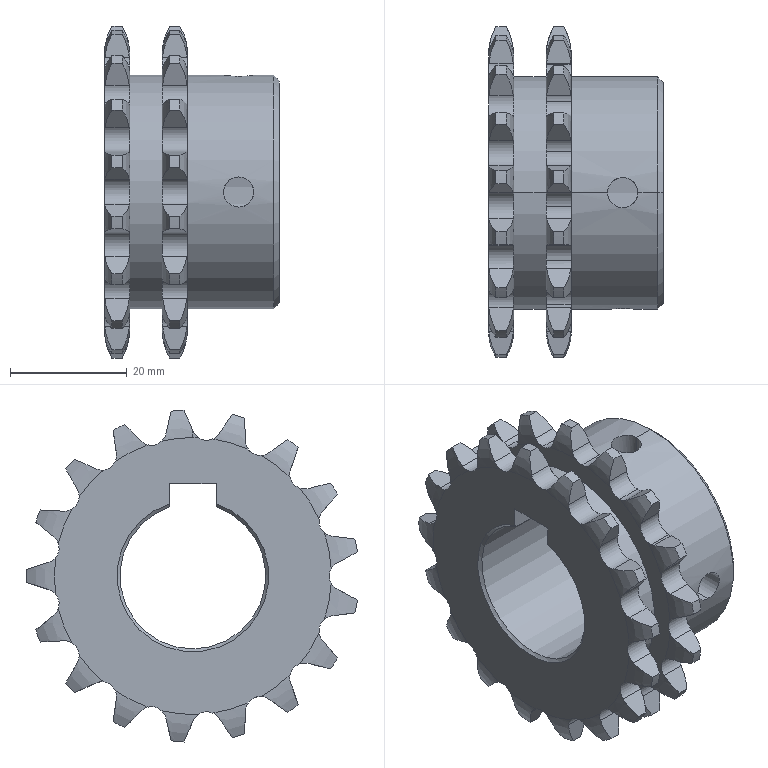Part | SolidWorks | features BaseBody 1 | 1 solid | 242 faces | box 30 x 56.698 x 56.919 mm | volume 28426 mm3 | cylinder 89 | plane 76 | spline 72 | cone 5 | commonest cylinder face diameters 5.08 x46 57 x34 5.188 x4 40 x4 25 x1